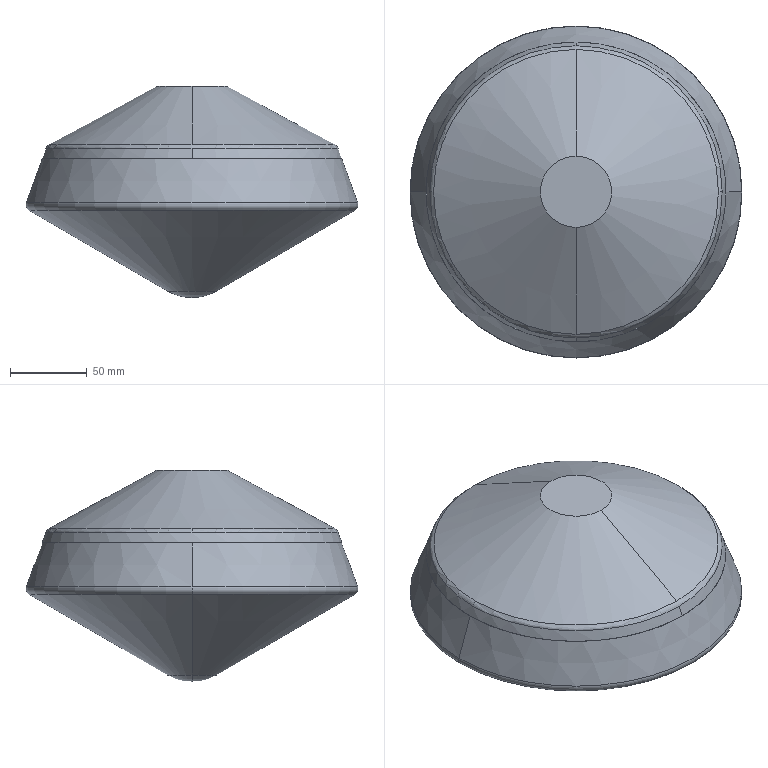Part | SolidWorks | features BaseBody 1, Revolution 1 | 2 solids | 17 faces | box 216.513 x 216.513 x 137.693 mm | volume 2586859 mm3 | cone 8 | torus 6 | plane 3
STEP:
#1=CARTESIAN_POINT('',(711.552,150.,-95.634));
#2=VERTEX_POINT('',#1);
#3=CARTESIAN_POINT('',(679.419,150.,-95.634));
#4=VERTEX_POINT('',#3);
#5=CARTESIAN_POINT('',(695.485,150.,-95.634));
#6=DIRECTION('',(0.,0.,1.));
#7=DIRECTION('',(1.,0.,0.));
#8=AXIS2_PLACEMENT_3D('',#5,#6,#7);
#9=CIRCLE('',#8,16.067);
#10=EDGE_CURVE('',#2,#4,#9,.T.);
#11=ORIENTED_EDGE('',*,*,#10,.T.);
#12=CARTESIAN_POINT('',(589.364,150.,-43.161));
#13=VERTEX_POINT('',#12);
#14=CARTESIAN_POINT('',(589.364,150.,-43.161));
#15=DIRECTION('',(-0.864,0.,0.5034));
#16=VECTOR('',#15,1000.);
#17=LINE('',#14,#16);
#18=EDGE_CURVE('',#4,#13,#17,.T.);
#19=ORIENTED_EDGE('',*,*,#18,.T.);
#20=CARTESIAN_POINT('',(801.607,150.,-43.161));
#21=VERTEX_POINT('',#20);
#22=CARTESIAN_POINT('',(695.485,150.,-43.161));
#23=DIRECTION('',(0.,0.,1.));
#24=DIRECTION('',(1.,0.,0.));
#25=AXIS2_PLACEMENT_3D('',#22,#23,#24);
#26=CIRCLE('',#25,106.121);
#27=EDGE_CURVE('',#21,#13,#26,.T.);
#28=ORIENTED_EDGE('',*,*,#27,.F.);
#29=CARTESIAN_POINT('',(801.607,150.,-43.161));
#30=DIRECTION('',(0.864,0.,0.5034));
#31=VECTOR('',#30,1000.);
#32=LINE('',#29,#31);
#33=EDGE_CURVE('',#2,#21,#32,.T.);
#34=ORIENTED_EDGE('',*,*,#33,.F.);
#35=EDGE_LOOP('',(#11,#19,#28,#34));
#36=FACE_OUTER_BOUND('',#35,.T.);
#37=CARTESIAN_POINT('',(695.485,150.,-43.161));
#38=DIRECTION('',(0.,0.,1.));
#39=DIRECTION('',(1.,0.,0.));
#40=AXIS2_PLACEMENT_3D('',#37,#38,#39);
#41=CONICAL_SURFACE('',#40,106.121,1.043);
#42=ADVANCED_FACE('',(#36),#41,.T.);
#43=ORIENTED_EDGE('',*,*,#27,.T.);
#44=CARTESIAN_POINT('',(587.485,150.,-37.983));
#45=VERTEX_POINT('',#44);
#46=CARTESIAN_POINT('',(591.529,150.,-39.446));
#47=DIRECTION('',(0.,1.,0.));
#48=DIRECTION('',(-1.,0.,0.));
#49=AXIS2_PLACEMENT_3D('',#46,#47,#48);
#50=CIRCLE('',#49,4.3);
#51=EDGE_CURVE('',#13,#45,#50,.T.);
#52=ORIENTED_EDGE('',*,*,#51,.T.);
#53=CARTESIAN_POINT('',(803.486,150.,-37.983));
#54=VERTEX_POINT('',#53);
#55=CARTESIAN_POINT('',(695.485,150.,-37.983));
#56=DIRECTION('',(0.,0.,1.));
#57=DIRECTION('',(1.,0.,0.));
#58=AXIS2_PLACEMENT_3D('',#55,#56,#57);
#59=CIRCLE('',#58,108.);
#60=EDGE_CURVE('',#54,#45,#59,.T.);
#61=ORIENTED_EDGE('',*,*,#60,.F.);
#62=CARTESIAN_POINT('',(799.442,150.,-39.446));
#63=DIRECTION('',(0.,-1.,0.));
#64=DIRECTION('',(0.,0.,-1.));
#65=AXIS2_PLACEMENT_3D('',#62,#63,#64);
#66=CIRCLE('',#65,4.3);
#67=EDGE_CURVE('',#21,#54,#66,.T.);
#68=ORIENTED_EDGE('',*,*,#67,.F.);
#69=EDGE_LOOP('',(#43,#52,#61,#68));
#70=FACE_OUTER_BOUND('',#69,.T.);
#71=CARTESIAN_POINT('',(695.485,150.,-39.446));
#72=DIRECTION('',(0.,0.,1.));
#73=DIRECTION('',(1.,0.,0.));
#74=AXIS2_PLACEMENT_3D('',#71,#72,#73);
#75=TOROIDAL_SURFACE('',#74,103.957,4.3);
#76=ADVANCED_FACE('',(#70),#75,.T.);
#77=CARTESIAN_POINT('',(793.196,150.,-9.535));
#78=VERTEX_POINT('',#77);
#79=CARTESIAN_POINT('',(597.775,150.,-9.535));
#80=VERTEX_POINT('',#79);
#81=CARTESIAN_POINT('',(695.485,150.,-9.535));
#82=DIRECTION('',(0.,0.,1.));
#83=DIRECTION('',(1.,0.,0.));
#84=AXIS2_PLACEMENT_3D('',#81,#82,#83);
#85=CIRCLE('',#84,97.711);
#86=EDGE_CURVE('',#78,#80,#85,.T.);
#87=ORIENTED_EDGE('',*,*,#86,.F.);
#88=CARTESIAN_POINT('',(793.196,150.,-9.535));
#89=DIRECTION('',(0.3401,0.,-0.9404));
#90=VECTOR('',#89,1000.);
#91=LINE('',#88,#90);
#92=EDGE_CURVE('',#78,#54,#91,.T.);
#93=ORIENTED_EDGE('',*,*,#92,.T.);
#94=ORIENTED_EDGE('',*,*,#60,.T.);
#95=CARTESIAN_POINT('',(597.775,150.,-9.535));
#96=DIRECTION('',(-0.3401,0.,-0.9404));
#97=VECTOR('',#96,1000.);
#98=LINE('',#95,#97);
#99=EDGE_CURVE('',#80,#45,#98,.T.);
#100=ORIENTED_EDGE('',*,*,#99,.F.);
#101=EDGE_LOOP('',(#87,#93,#94,#100));
#102=FACE_OUTER_BOUND('',#101,.T.);
#103=CARTESIAN_POINT('',(695.485,150.,-9.535));
#104=DIRECTION('',(0.,0.,-1.));
#105=DIRECTION('',(-1.,0.,0.));
#106=AXIS2_PLACEMENT_3D('',#103,#104,#105);
#107=CONICAL_SURFACE('',#106,97.711,0.3471);
#108=ADVANCED_FACE('',(#102),#107,.T.);
#109=CARTESIAN_POINT('',(695.485,150.,-99.928));
#110=VERTEX_POINT('',#109);
#111=CARTESIAN_POINT('',(695.651,150.,-68.344));
#112=DIRECTION('',(0.,-1.,0.));
#113=DIRECTION('',(0.,0.,-1.));
#114=AXIS2_PLACEMENT_3D('',#111,#112,#113);
#115=CIRCLE('',#114,31.584);
#116=EDGE_CURVE('',#110,#2,#115,.T.);
#117=ORIENTED_EDGE('',*,*,#116,.F.);
#118=CARTESIAN_POINT('',(695.319,150.,-68.344));
#119=DIRECTION('',(0.,1.,0.));
#120=DIRECTION('',(-1.,0.,0.));
#121=AXIS2_PLACEMENT_3D('',#118,#119,#120);
#122=CIRCLE('',#121,31.584);
#123=EDGE_CURVE('',#110,#4,#122,.T.);
#124=ORIENTED_EDGE('',*,*,#123,.T.);
#125=ORIENTED_EDGE('',*,*,#10,.F.);
#126=EDGE_LOOP('',(#117,#124,#125));
#127=FACE_OUTER_BOUND('',#126,.T.);
#128=CARTESIAN_POINT('',(695.485,150.,-68.344));
#129=DIRECTION('',(0.,0.,1.));
#130=DIRECTION('',(1.,0.,0.));
#131=AXIS2_PLACEMENT_3D('',#128,#129,#130);
#132=TOROIDAL_SURFACE('',#131,0.166,31.584);
#133=ADVANCED_FACE('',(#127),#132,.T.);
#134=ORIENTED_EDGE('',*,*,#123,.F.);
#135=ORIENTED_EDGE('',*,*,#116,.T.);
#136=CARTESIAN_POINT('',(695.485,150.,-95.634));
#137=DIRECTION('',(0.,0.,1.));
#138=DIRECTION('',(1.,0.,0.));
#139=AXIS2_PLACEMENT_3D('',#136,#137,#138);
#140=CIRCLE('',#139,16.067);
#141=EDGE_CURVE('',#4,#2,#140,.T.);
#142=ORIENTED_EDGE('',*,*,#141,.F.);
#143=EDGE_LOOP('',(#134,#135,#142));
#144=FACE_OUTER_BOUND('',#143,.T.);
#145=CARTESIAN_POINT('',(695.485,150.,-68.344));
#146=DIRECTION('',(0.,0.,1.));
#147=DIRECTION('',(1.,0.,0.));
#148=AXIS2_PLACEMENT_3D('',#145,#146,#147);
#149=TOROIDAL_SURFACE('',#148,0.166,31.584);
#150=ADVANCED_FACE('',(#144),#149,.T.);
#151=CARTESIAN_POINT('',(695.485,150.,-9.535));
#152=DIRECTION('',(0.,0.,1.));
#153=DIRECTION('',(1.,0.,0.));
#154=AXIS2_PLACEMENT_3D('',#151,#152,#153);
#155=CIRCLE('',#154,97.711);
#156=EDGE_CURVE('',#80,#78,#155,.T.);
#157=ORIENTED_EDGE('',*,*,#156,.T.);
#158=ORIENTED_EDGE('',*,*,#86,.T.);
#159=EDGE_LOOP('',(#157,#158));
#160=FACE_OUTER_BOUND('',#159,.T.);
#161=CARTESIAN_POINT('',(695.485,150.,-9.535));
#162=DIRECTION('',(0.,0.,1.));
#163=DIRECTION('',(1.,0.,0.));
#164=AXIS2_PLACEMENT_3D('',#161,#162,#163);
#165=PLANE('',#164);
#166=ADVANCED_FACE('',(#160),#165,.T.);
#167=ORIENTED_EDGE('',*,*,#92,.F.);
#168=ORIENTED_EDGE('',*,*,#156,.F.);
#169=ORIENTED_EDGE('',*,*,#99,.T.);
#170=CARTESIAN_POINT('',(695.485,150.,-37.983));
#171=DIRECTION('',(0.,0.,1.));
#172=DIRECTION('',(1.,0.,0.));
#173=AXIS2_PLACEMENT_3D('',#170,#171,#172);
#174=CIRCLE('',#173,108.);
#175=EDGE_CURVE('',#45,#54,#174,.T.);
#176=ORIENTED_EDGE('',*,*,#175,.T.);
#177=EDGE_LOOP('',(#167,#168,#169,#176));
#178=FACE_OUTER_BOUND('',#177,.T.);
#179=CARTESIAN_POINT('',(695.485,150.,-9.535));
#180=DIRECTION('',(0.,0.,-1.));
#181=DIRECTION('',(-1.,0.,0.));
#182=AXIS2_PLACEMENT_3D('',#179,#180,#181);
#183=CONICAL_SURFACE('',#182,97.711,0.3471);
#184=ADVANCED_FACE('',(#178),#183,.T.);
#185=ORIENTED_EDGE('',*,*,#51,.F.);
#186=CARTESIAN_POINT('',(695.485,150.,-43.161));
#187=DIRECTION('',(0.,0.,1.));
#188=DIRECTION('',(1.,0.,0.));
#189=AXIS2_PLACEMENT_3D('',#186,#187,#188);
#190=CIRCLE('',#189,106.121);
#191=EDGE_CURVE('',#13,#21,#190,.T.);
#192=ORIENTED_EDGE('',*,*,#191,.T.);
#193=ORIENTED_EDGE('',*,*,#67,.T.);
#194=ORIENTED_EDGE('',*,*,#175,.F.);
#195=EDGE_LOOP('',(#185,#192,#193,#194));
#196=FACE_OUTER_BOUND('',#195,.T.);
#197=CARTESIAN_POINT('',(695.485,150.,-39.446));
#198=DIRECTION('',(0.,0.,1.));
#199=DIRECTION('',(1.,0.,0.));
#200=AXIS2_PLACEMENT_3D('',#197,#198,#199);
#201=TOROIDAL_SURFACE('',#200,103.957,4.3);
#202=ADVANCED_FACE('',(#196),#201,.T.);
#203=ORIENTED_EDGE('',*,*,#18,.F.);
#204=ORIENTED_EDGE('',*,*,#141,.T.);
#205=ORIENTED_EDGE('',*,*,#33,.T.);
#206=ORIENTED_EDGE('',*,*,#191,.F.);
#207=EDGE_LOOP('',(#203,#204,#205,#206));
#208=FACE_OUTER_BOUND('',#207,.T.);
#209=CARTESIAN_POINT('',(695.485,150.,-43.161));
#210=DIRECTION('',(0.,0.,1.));
#211=DIRECTION('',(1.,0.,0.));
#212=AXIS2_PLACEMENT_3D('',#209,#210,#211);
#213=CONICAL_SURFACE('',#212,106.121,1.043);
#214=ADVANCED_FACE('',(#208),#213,.T.);
#215=CLOSED_SHELL('',(#42,#76,#108,#133,#150,#166,#184,#202,#214));
#216=MANIFOLD_SOLID_BREP('',#215);
#217=CARTESIAN_POINT('',(695.485,57.125,0.));
#218=VERTEX_POINT('',#217);
#219=CARTESIAN_POINT('',(602.611,150.,0.));
#220=VERTEX_POINT('',#219);
#221=CARTESIAN_POINT('',(695.485,150.,0.));
#222=DIRECTION('',(0.,0.,-1.));
#223=DIRECTION('',(0.,1.,0.));
#224=AXIS2_PLACEMENT_3D('',#221,#222,#223);
#225=CIRCLE('',#224,92.875);
#226=EDGE_CURVE('',#218,#220,#225,.T.);
#227=ORIENTED_EDGE('',*,*,#226,.T.);
#228=CARTESIAN_POINT('',(600.218,150.,-2.781));
#229=VERTEX_POINT('',#228);
#230=CARTESIAN_POINT('',(605.07,150.,-4.536));
#231=DIRECTION('',(0.,-1.,0.));
#232=DIRECTION('',(1.,0.,0.));
#233=AXIS2_PLACEMENT_3D('',#230,#231,#232);
#234=CIRCLE('',#233,5.16);
#235=EDGE_CURVE('',#220,#229,#234,.T.);
#236=ORIENTED_EDGE('',*,*,#235,.T.);
#237=CARTESIAN_POINT('',(695.485,54.732,-2.781));
#238=VERTEX_POINT('',#237);
#239=CARTESIAN_POINT('',(695.485,150.,-2.781));
#240=DIRECTION('',(0.,0.,1.));
#241=DIRECTION('',(0.,1.,0.));
#242=AXIS2_PLACEMENT_3D('',#239,#240,#241);
#243=CIRCLE('',#242,95.268);
#244=EDGE_CURVE('',#229,#238,#243,.T.);
#245=ORIENTED_EDGE('',*,*,#244,.T.);
#246=CARTESIAN_POINT('',(790.753,150.,-2.781));
#247=VERTEX_POINT('',#246);
#248=CARTESIAN_POINT('',(695.485,150.,-2.781));
#249=DIRECTION('',(0.,0.,1.));
#250=DIRECTION('',(0.,1.,0.));
#251=AXIS2_PLACEMENT_3D('',#248,#249,#250);
#252=CIRCLE('',#251,95.268);
#253=EDGE_CURVE('',#238,#247,#252,.T.);
#254=ORIENTED_EDGE('',*,*,#253,.T.);
#255=CARTESIAN_POINT('',(788.36,150.,0.));
#256=VERTEX_POINT('',#255);
#257=CARTESIAN_POINT('',(785.901,150.,-4.536));
#258=DIRECTION('',(0.,1.,0.));
#259=DIRECTION('',(0.,0.,1.));
#260=AXIS2_PLACEMENT_3D('',#257,#258,#259);
#261=CIRCLE('',#260,5.16);
#262=EDGE_CURVE('',#256,#247,#261,.T.);
#263=ORIENTED_EDGE('',*,*,#262,.F.);
#264=CARTESIAN_POINT('',(695.485,150.,0.));
#265=DIRECTION('',(0.,0.,-1.));
#266=DIRECTION('',(0.,1.,0.));
#267=AXIS2_PLACEMENT_3D('',#264,#265,#266);
#268=CIRCLE('',#267,92.875);
#269=EDGE_CURVE('',#256,#218,#268,.T.);
#270=ORIENTED_EDGE('',*,*,#269,.T.);
#271=EDGE_LOOP('',(#227,#236,#245,#254,#263,#270));
#272=FACE_OUTER_BOUND('',#271,.T.);
#273=CARTESIAN_POINT('',(695.485,150.,-4.536));
#274=DIRECTION('',(0.,0.,-1.));
#275=DIRECTION('',(1.,0.,0.));
#276=AXIS2_PLACEMENT_3D('',#273,#274,#275);
#277=TOROIDAL_SURFACE('',#276,90.415,5.16);
#278=ADVANCED_FACE('',(#272),#277,.T.);
#279=CARTESIAN_POINT('',(695.485,245.268,-2.781));
#280=VERTEX_POINT('',#279);
#281=CARTESIAN_POINT('',(695.485,150.,-2.781));
#282=DIRECTION('',(0.,0.,1.));
#283=DIRECTION('',(0.,1.,0.));
#284=AXIS2_PLACEMENT_3D('',#281,#282,#283);
#285=CIRCLE('',#284,95.268);
#286=EDGE_CURVE('',#280,#229,#285,.T.);
#287=ORIENTED_EDGE('',*,*,#286,.F.);
#288=CARTESIAN_POINT('',(695.485,247.711,-9.535));
#289=VERTEX_POINT('',#288);
#290=CARTESIAN_POINT('',(695.485,251.91,-21.145));
#291=DIRECTION('',(0.,0.3401,-0.9404));
#292=VECTOR('',#291,1000.);
#293=LINE('',#290,#292);
#294=EDGE_CURVE('',#280,#289,#293,.T.);
#295=ORIENTED_EDGE('',*,*,#294,.T.);
#296=CARTESIAN_POINT('',(695.485,52.289,-9.535));
#297=VERTEX_POINT('',#296);
#298=CARTESIAN_POINT('',(695.485,150.,-9.535));
#299=DIRECTION('',(0.,0.,1.));
#300=DIRECTION('',(0.,-1.,0.));
#301=AXIS2_PLACEMENT_3D('',#298,#299,#300);
#302=CIRCLE('',#301,97.711);
#303=EDGE_CURVE('',#289,#297,#302,.T.);
#304=ORIENTED_EDGE('',*,*,#303,.T.);
#305=CARTESIAN_POINT('',(695.485,48.09,-21.145));
#306=DIRECTION('',(0.,-0.3401,-0.9404));
#307=VECTOR('',#306,1000.);
#308=LINE('',#305,#307);
#309=EDGE_CURVE('',#238,#297,#308,.T.);
#310=ORIENTED_EDGE('',*,*,#309,.F.);
#311=ORIENTED_EDGE('',*,*,#244,.F.);
#312=EDGE_LOOP('',(#287,#295,#304,#310,#311));
#313=FACE_OUTER_BOUND('',#312,.T.);
#314=CARTESIAN_POINT('',(695.485,150.,-21.145));
#315=DIRECTION('',(0.,0.,-1.));
#316=DIRECTION('',(0.,-1.,0.));
#317=AXIS2_PLACEMENT_3D('',#314,#315,#316);
#318=CONICAL_SURFACE('',#317,101.91,0.3471);
#319=ADVANCED_FACE('',(#313),#318,.T.);
#320=CARTESIAN_POINT('',(695.485,126.78,37.765));
#321=VERTEX_POINT('',#320);
#322=CARTESIAN_POINT('',(695.485,173.22,37.765));
#323=VERTEX_POINT('',#322);
#324=CARTESIAN_POINT('',(695.485,150.,37.765));
#325=DIRECTION('',(0.,0.,-1.));
#326=DIRECTION('',(-1.,0.,0.));
#327=AXIS2_PLACEMENT_3D('',#324,#325,#326);
#328=CIRCLE('',#327,23.22);
#329=EDGE_CURVE('',#321,#323,#328,.T.);
#330=ORIENTED_EDGE('',*,*,#329,.T.);
#331=CARTESIAN_POINT('',(695.485,242.875,0.));
#332=VERTEX_POINT('',#331);
#333=CARTESIAN_POINT('',(695.485,208.91,18.415));
#334=DIRECTION('',(0.,0.8791,-0.4766));
#335=VECTOR('',#334,1000.);
#336=LINE('',#333,#335);
#337=EDGE_CURVE('',#323,#332,#336,.T.);
#338=ORIENTED_EDGE('',*,*,#337,.T.);
#339=CARTESIAN_POINT('',(695.485,150.,0.));
#340=DIRECTION('',(0.,0.,-1.));
#341=DIRECTION('',(0.,1.,0.));
#342=AXIS2_PLACEMENT_3D('',#339,#340,#341);
#343=CIRCLE('',#342,92.875);
#344=EDGE_CURVE('',#220,#332,#343,.T.);
#345=ORIENTED_EDGE('',*,*,#344,.F.);
#346=ORIENTED_EDGE('',*,*,#226,.F.);
#347=CARTESIAN_POINT('',(695.485,91.09,18.415));
#348=DIRECTION('',(0.,-0.8791,-0.4766));
#349=VECTOR('',#348,1000.);
#350=LINE('',#347,#349);
#351=EDGE_CURVE('',#321,#218,#350,.T.);
#352=ORIENTED_EDGE('',*,*,#351,.F.);
#353=EDGE_LOOP('',(#330,#338,#345,#346,#352));
#354=FACE_OUTER_BOUND('',#353,.T.);
#355=CARTESIAN_POINT('',(695.485,150.,18.415));
#356=DIRECTION('',(0.,0.,-1.));
#357=DIRECTION('',(0.,-1.,0.));
#358=AXIS2_PLACEMENT_3D('',#355,#356,#357);
#359=CONICAL_SURFACE('',#358,58.91,1.074);
#360=ADVANCED_FACE('',(#354),#359,.T.);
#361=ORIENTED_EDGE('',*,*,#329,.F.);
#362=CARTESIAN_POINT('',(695.485,150.,37.765));
#363=DIRECTION('',(0.,0.,-1.));
#364=DIRECTION('',(-1.,0.,0.));
#365=AXIS2_PLACEMENT_3D('',#362,#363,#364);
#366=CIRCLE('',#365,23.22);
#367=EDGE_CURVE('',#323,#321,#366,.T.);
#368=ORIENTED_EDGE('',*,*,#367,.F.);
#369=EDGE_LOOP('',(#361,#368));
#370=FACE_OUTER_BOUND('',#369,.T.);
#371=CARTESIAN_POINT('',(695.485,126.78,37.765));
#372=DIRECTION('',(0.,0.,1.));
#373=DIRECTION('',(1.,0.,0.));
#374=AXIS2_PLACEMENT_3D('',#371,#372,#373);
#375=PLANE('',#374);
#376=ADVANCED_FACE('',(#370),#375,.T.);
#377=ORIENTED_EDGE('',*,*,#337,.F.);
#378=ORIENTED_EDGE('',*,*,#367,.T.);
#379=ORIENTED_EDGE('',*,*,#351,.T.);
#380=ORIENTED_EDGE('',*,*,#269,.F.);
#381=CARTESIAN_POINT('',(695.485,150.,0.));
#382=DIRECTION('',(0.,0.,-1.));
#383=DIRECTION('',(0.,1.,0.));
#384=AXIS2_PLACEMENT_3D('',#381,#382,#383);
#385=CIRCLE('',#384,92.875);
#386=EDGE_CURVE('',#332,#256,#385,.T.);
#387=ORIENTED_EDGE('',*,*,#386,.F.);
#388=EDGE_LOOP('',(#377,#378,#379,#380,#387));
#389=FACE_OUTER_BOUND('',#388,.T.);
#390=CARTESIAN_POINT('',(695.485,150.,18.415));
#391=DIRECTION('',(0.,0.,-1.));
#392=DIRECTION('',(0.,-1.,0.));
#393=AXIS2_PLACEMENT_3D('',#390,#391,#392);
#394=CONICAL_SURFACE('',#393,58.91,1.074);
#395=ADVANCED_FACE('',(#389),#394,.T.);
#396=ORIENTED_EDGE('',*,*,#294,.F.);
#397=CARTESIAN_POINT('',(695.485,150.,-2.781));
#398=DIRECTION('',(0.,0.,1.));
#399=DIRECTION('',(0.,1.,0.));
#400=AXIS2_PLACEMENT_3D('',#397,#398,#399);
#401=CIRCLE('',#400,95.268);
#402=EDGE_CURVE('',#247,#280,#401,.T.);
#403=ORIENTED_EDGE('',*,*,#402,.F.);
#404=ORIENTED_EDGE('',*,*,#253,.F.);
#405=ORIENTED_EDGE('',*,*,#309,.T.);
#406=CARTESIAN_POINT('',(695.485,150.,-9.535));
#407=DIRECTION('',(0.,0.,1.));
#408=DIRECTION('',(0.,-1.,0.));
#409=AXIS2_PLACEMENT_3D('',#406,#407,#408);
#410=CIRCLE('',#409,97.711);
#411=EDGE_CURVE('',#297,#289,#410,.T.);
#412=ORIENTED_EDGE('',*,*,#411,.T.);
#413=EDGE_LOOP('',(#396,#403,#404,#405,#412));
#414=FACE_OUTER_BOUND('',#413,.T.);
#415=CARTESIAN_POINT('',(695.485,150.,-21.145));
#416=DIRECTION('',(0.,0.,-1.));
#417=DIRECTION('',(0.,-1.,0.));
#418=AXIS2_PLACEMENT_3D('',#415,#416,#417);
#419=CONICAL_SURFACE('',#418,101.91,0.3471);
#420=ADVANCED_FACE('',(#414),#419,.T.);
#421=ORIENTED_EDGE('',*,*,#235,.F.);
#422=ORIENTED_EDGE('',*,*,#344,.T.);
#423=ORIENTED_EDGE('',*,*,#386,.T.);
#424=ORIENTED_EDGE('',*,*,#262,.T.);
#425=ORIENTED_EDGE('',*,*,#402,.T.);
#426=ORIENTED_EDGE('',*,*,#286,.T.);
#427=EDGE_LOOP('',(#421,#422,#423,#424,#425,#426));
#428=FACE_OUTER_BOUND('',#427,.T.);
#429=CARTESIAN_POINT('',(695.485,150.,-4.536));
#430=DIRECTION('',(0.,0.,-1.));
#431=DIRECTION('',(1.,0.,0.));
#432=AXIS2_PLACEMENT_3D('',#429,#430,#431);
#433=TOROIDAL_SURFACE('',#432,90.415,5.16);
#434=ADVANCED_FACE('',(#428),#433,.T.);
#435=ORIENTED_EDGE('',*,*,#411,.F.);
#436=ORIENTED_EDGE('',*,*,#303,.F.);
#437=EDGE_LOOP('',(#435,#436));
#438=FACE_OUTER_BOUND('',#437,.T.);
#439=CARTESIAN_POINT('',(695.485,150.,-9.535));
#440=DIRECTION('',(0.,0.,1.));
#441=DIRECTION('',(1.,0.,0.));
#442=AXIS2_PLACEMENT_3D('',#439,#440,#441);
#443=PLANE('',#442);
#444=ADVANCED_FACE('',(#438),#443,.F.);
#445=CLOSED_SHELL('',(#278,#319,#360,#376,#395,#420,#434,#444));
#446=MANIFOLD_SOLID_BREP('',#445);
#447=CARTESIAN_POINT('',(0.,0.,0.));
#448=DIRECTION('',(0.,0.,1.));
#449=DIRECTION('',(1.,0.,0.));
#450=AXIS2_PLACEMENT_3D('',#447,#448,#449);
#451=(LENGTH_UNIT()NAMED_UNIT(*)SI_UNIT(.MILLI.,.METRE.));
#452=UNCERTAINTY_MEASURE_WITH_UNIT(LENGTH_MEASURE(0.00001),#451,'','');
#453=(NAMED_UNIT(*)PLANE_ANGLE_UNIT()SI_UNIT($,.RADIAN.));
#454=(NAMED_UNIT(*)SI_UNIT($,.STERADIAN.)SOLID_ANGLE_UNIT());
#455=(GEOMETRIC_REPRESENTATION_CONTEXT(3)GLOBAL_UNCERTAINTY_ASSIGNED_CONTEXT((#452))GLOBAL_UNIT_ASSIGNED_CONTEXT((#451,#453,#454))REPRESENTATION_CONTEXT('',''));
#456=ADVANCED_BREP_SHAPE_REPRESENTATION('',(#216,#446,#450),#455);